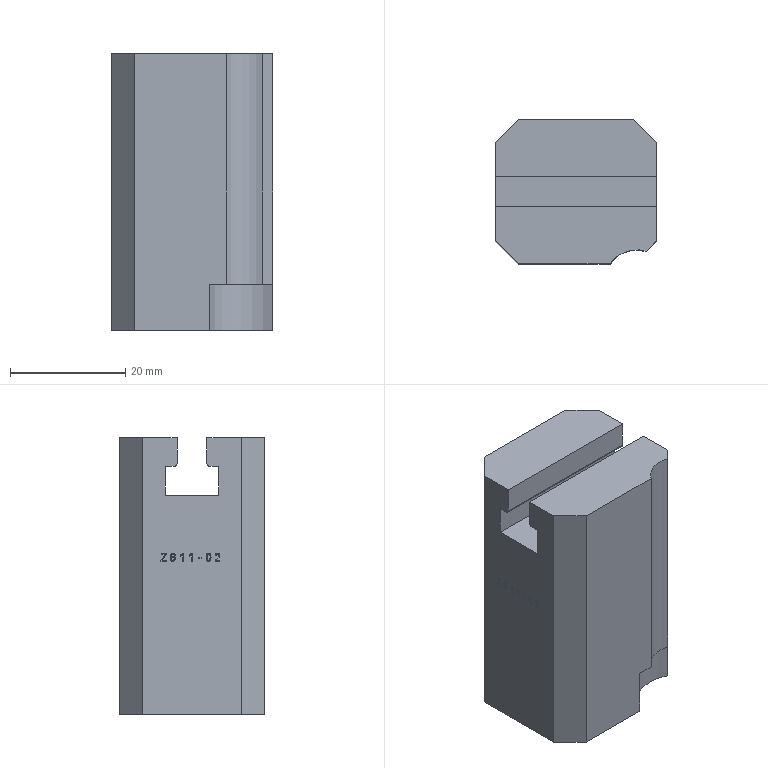Part | Creo | 1 solid | 143 faces | box 28 x 25 x 48 mm | volume 27587 mm3 | other 77 | plane 54 | cylinder 10 | cone 2 | commonest cylinder face diameters 1 x2 8.499 x2 8.5 x2 1.208 x1 11 x1 16 x1